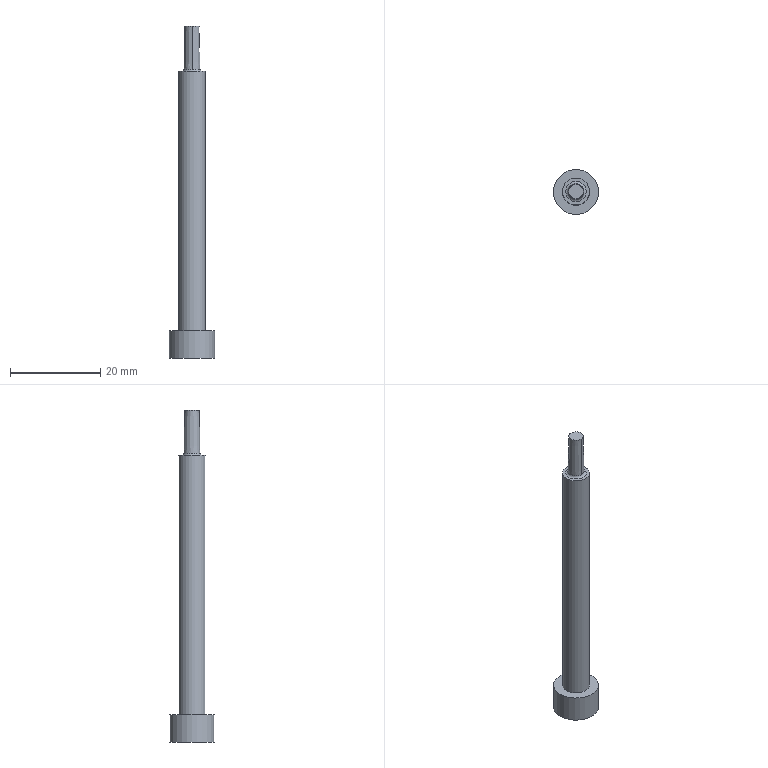Part | STEP file | solid 2 | 1 solid | 9 faces | box 10 x 10 x 73.694 mm | volume 2193 mm3 | plane 4 | cylinder 2 | cone 2 | torus 1 | commonest cylinder face diameters 6 x1 10 x1